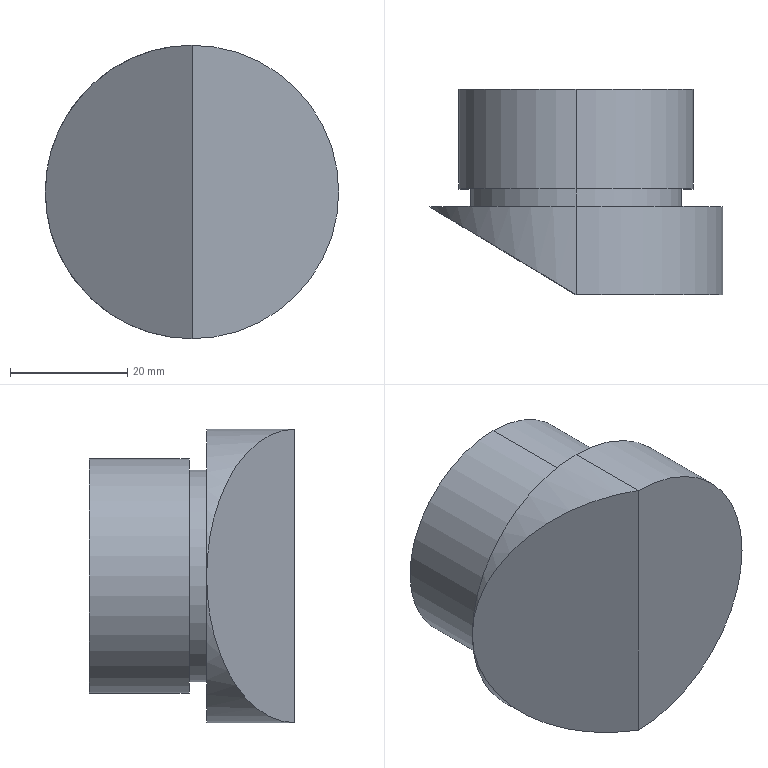Part | SolidWorks | features ICE 1, Revolution 1 | 1 solid | 12 faces | box 50 x 35 x 50 mm | volume 47619 mm3 | cylinder 7 | plane 5 | commonest cylinder face diameters 50 x3 36 x2 40 x2
STEP:
#1=CARTESIAN_POINT('',(0.,-2.175,18.));
#2=VERTEX_POINT('',#1);
#3=CARTESIAN_POINT('',(0.,-2.175,-18.));
#4=VERTEX_POINT('',#3);
#5=CARTESIAN_POINT('',(0.,-2.175,0.));
#6=DIRECTION('',(0.,1.,0.));
#7=DIRECTION('',(0.,0.,1.));
#8=AXIS2_PLACEMENT_3D('',#5,#6,#7);
#9=CIRCLE('',#8,18.);
#10=EDGE_CURVE('',#2,#4,#9,.T.);
#11=ORIENTED_EDGE('',*,*,#10,.T.);
#12=CARTESIAN_POINT('',(0.,0.8255,-18.));
#13=VERTEX_POINT('',#12);
#14=CARTESIAN_POINT('',(0.,13.712,-18.));
#15=DIRECTION('',(0.,1.,0.));
#16=VECTOR('',#15,1000.);
#17=LINE('',#14,#16);
#18=EDGE_CURVE('',#4,#13,#17,.T.);
#19=ORIENTED_EDGE('',*,*,#18,.T.);
#20=CARTESIAN_POINT('',(0.,0.8255,18.));
#21=VERTEX_POINT('',#20);
#22=CARTESIAN_POINT('',(0.,0.8255,0.));
#23=DIRECTION('',(0.,1.,0.));
#24=DIRECTION('',(0.,0.,1.));
#25=AXIS2_PLACEMENT_3D('',#22,#23,#24);
#26=CIRCLE('',#25,18.);
#27=EDGE_CURVE('',#21,#13,#26,.T.);
#28=ORIENTED_EDGE('',*,*,#27,.F.);
#29=CARTESIAN_POINT('',(0.,13.712,18.));
#30=DIRECTION('',(0.,1.,0.));
#31=VECTOR('',#30,1000.);
#32=LINE('',#29,#31);
#33=EDGE_CURVE('',#2,#21,#32,.T.);
#34=ORIENTED_EDGE('',*,*,#33,.F.);
#35=EDGE_LOOP('',(#11,#19,#28,#34));
#36=FACE_OUTER_BOUND('',#35,.T.);
#37=CARTESIAN_POINT('',(0.,13.712,0.));
#38=DIRECTION('',(0.,1.,0.));
#39=DIRECTION('',(0.,0.,1.));
#40=AXIS2_PLACEMENT_3D('',#37,#38,#39);
#41=CYLINDRICAL_SURFACE('',#40,18.);
#42=ADVANCED_FACE('',(#36),#41,.T.);
#43=CARTESIAN_POINT('',(0.,0.8255,20.));
#44=VERTEX_POINT('',#43);
#45=CARTESIAN_POINT('',(0.,0.8255,-20.));
#46=VERTEX_POINT('',#45);
#47=CARTESIAN_POINT('',(0.,0.8255,0.));
#48=DIRECTION('',(0.,1.,0.));
#49=DIRECTION('',(0.,0.,1.));
#50=AXIS2_PLACEMENT_3D('',#47,#48,#49);
#51=CIRCLE('',#50,20.);
#52=EDGE_CURVE('',#44,#46,#51,.T.);
#53=ORIENTED_EDGE('',*,*,#52,.T.);
#54=CARTESIAN_POINT('',(0.,17.825,-20.));
#55=VERTEX_POINT('',#54);
#56=CARTESIAN_POINT('',(0.,13.712,-20.));
#57=DIRECTION('',(0.,1.,0.));
#58=VECTOR('',#57,1000.);
#59=LINE('',#56,#58);
#60=EDGE_CURVE('',#46,#55,#59,.T.);
#61=ORIENTED_EDGE('',*,*,#60,.T.);
#62=CARTESIAN_POINT('',(0.,17.825,20.));
#63=VERTEX_POINT('',#62);
#64=CARTESIAN_POINT('',(0.,17.825,0.));
#65=DIRECTION('',(0.,1.,0.));
#66=DIRECTION('',(0.,0.,1.));
#67=AXIS2_PLACEMENT_3D('',#64,#65,#66);
#68=CIRCLE('',#67,20.);
#69=EDGE_CURVE('',#63,#55,#68,.T.);
#70=ORIENTED_EDGE('',*,*,#69,.F.);
#71=CARTESIAN_POINT('',(0.,13.712,20.));
#72=DIRECTION('',(0.,1.,0.));
#73=VECTOR('',#72,1000.);
#74=LINE('',#71,#73);
#75=EDGE_CURVE('',#44,#63,#74,.T.);
#76=ORIENTED_EDGE('',*,*,#75,.F.);
#77=EDGE_LOOP('',(#53,#61,#70,#76));
#78=FACE_OUTER_BOUND('',#77,.T.);
#79=CARTESIAN_POINT('',(0.,13.712,0.));
#80=DIRECTION('',(0.,1.,0.));
#81=DIRECTION('',(0.,0.,1.));
#82=AXIS2_PLACEMENT_3D('',#79,#80,#81);
#83=CYLINDRICAL_SURFACE('',#82,20.);
#84=ADVANCED_FACE('',(#78),#83,.T.);
#85=CARTESIAN_POINT('',(0.,-17.175,25.));
#86=VERTEX_POINT('',#85);
#87=CARTESIAN_POINT('',(0.,-17.175,-25.));
#88=VERTEX_POINT('',#87);
#89=CARTESIAN_POINT('',(0.,-17.175,0.));
#90=DIRECTION('',(0.,1.,0.));
#91=DIRECTION('',(0.,0.,1.));
#92=AXIS2_PLACEMENT_3D('',#89,#90,#91);
#93=CIRCLE('',#92,25.);
#94=EDGE_CURVE('',#86,#88,#93,.T.);
#95=ORIENTED_EDGE('',*,*,#94,.T.);
#96=CARTESIAN_POINT('',(0.,-2.175,-25.));
#97=VERTEX_POINT('',#96);
#98=CARTESIAN_POINT('',(0.,13.712,-25.));
#99=DIRECTION('',(0.,1.,0.));
#100=VECTOR('',#99,1000.);
#101=LINE('',#98,#100);
#102=EDGE_CURVE('',#88,#97,#101,.T.);
#103=ORIENTED_EDGE('',*,*,#102,.T.);
#104=CARTESIAN_POINT('',(0.,-2.175,25.));
#105=VERTEX_POINT('',#104);
#106=CARTESIAN_POINT('',(0.,-2.175,0.));
#107=DIRECTION('',(0.,1.,0.));
#108=DIRECTION('',(0.,0.,1.));
#109=AXIS2_PLACEMENT_3D('',#106,#107,#108);
#110=CIRCLE('',#109,25.);
#111=EDGE_CURVE('',#105,#97,#110,.T.);
#112=ORIENTED_EDGE('',*,*,#111,.F.);
#113=CARTESIAN_POINT('',(0.,13.712,25.));
#114=DIRECTION('',(0.,1.,0.));
#115=VECTOR('',#114,1000.);
#116=LINE('',#113,#115);
#117=EDGE_CURVE('',#86,#105,#116,.T.);
#118=ORIENTED_EDGE('',*,*,#117,.F.);
#119=EDGE_LOOP('',(#95,#103,#112,#118));
#120=FACE_OUTER_BOUND('',#119,.T.);
#121=CARTESIAN_POINT('',(0.,13.712,0.));
#122=DIRECTION('',(0.,1.,0.));
#123=DIRECTION('',(0.,0.,1.));
#124=AXIS2_PLACEMENT_3D('',#121,#122,#123);
#125=CYLINDRICAL_SURFACE('',#124,25.);
#126=ADVANCED_FACE('',(#120),#125,.T.);
#127=CARTESIAN_POINT('',(-25.,-2.175,0.));
#128=VERTEX_POINT('',#127);
#129=CARTESIAN_POINT('',(-25.,-2.175,0.));
#130=CARTESIAN_POINT('',(-25.,-2.175,14.645));
#131=CARTESIAN_POINT('',(-14.645,-8.388,25.));
#132=CARTESIAN_POINT('',(0.,-17.175,25.));
#133=(BOUNDED_CURVE()B_SPLINE_CURVE(3,(#129,#130,#131,#132),.UNSPECIFIED.,.F.,.F.)B_SPLINE_CURVE_WITH_KNOTS((4,4),(0.,1.571),.UNSPECIFIED.)CURVE()GEOMETRIC_REPRESENTATION_ITEM()RATIONAL_B_SPLINE_CURVE((1.,0.8047,0.8047,1.))REPRESENTATION_ITEM(''));
#134=EDGE_CURVE('',#128,#86,#133,.T.);
#135=ORIENTED_EDGE('',*,*,#134,.T.);
#136=ORIENTED_EDGE('',*,*,#117,.T.);
#137=CARTESIAN_POINT('',(0.,-2.175,0.));
#138=DIRECTION('',(0.,1.,0.));
#139=DIRECTION('',(0.,0.,1.));
#140=AXIS2_PLACEMENT_3D('',#137,#138,#139);
#141=CIRCLE('',#140,25.);
#142=EDGE_CURVE('',#128,#105,#141,.T.);
#143=ORIENTED_EDGE('',*,*,#142,.F.);
#144=EDGE_LOOP('',(#135,#136,#143));
#145=FACE_OUTER_BOUND('',#144,.T.);
#146=CARTESIAN_POINT('',(0.,13.712,0.));
#147=DIRECTION('',(0.,1.,0.));
#148=DIRECTION('',(0.,0.,1.));
#149=AXIS2_PLACEMENT_3D('',#146,#147,#148);
#150=CYLINDRICAL_SURFACE('',#149,25.);
#151=ADVANCED_FACE('',(#145),#150,.T.);
#152=ORIENTED_EDGE('',*,*,#102,.F.);
#153=CARTESIAN_POINT('',(0.,-17.175,-25.));
#154=CARTESIAN_POINT('',(-14.645,-8.388,-25.));
#155=CARTESIAN_POINT('',(-25.,-2.175,-14.645));
#156=CARTESIAN_POINT('',(-25.,-2.175,0.));
#157=(BOUNDED_CURVE()B_SPLINE_CURVE(3,(#153,#154,#155,#156),.UNSPECIFIED.,.F.,.F.)B_SPLINE_CURVE_WITH_KNOTS((4,4),(4.712,6.283),.UNSPECIFIED.)CURVE()GEOMETRIC_REPRESENTATION_ITEM()RATIONAL_B_SPLINE_CURVE((1.,0.8047,0.8047,1.))REPRESENTATION_ITEM(''));
#158=EDGE_CURVE('',#88,#128,#157,.T.);
#159=ORIENTED_EDGE('',*,*,#158,.T.);
#160=CARTESIAN_POINT('',(0.,-2.175,0.));
#161=DIRECTION('',(0.,1.,0.));
#162=DIRECTION('',(0.,0.,1.));
#163=AXIS2_PLACEMENT_3D('',#160,#161,#162);
#164=CIRCLE('',#163,25.);
#165=EDGE_CURVE('',#97,#128,#164,.T.);
#166=ORIENTED_EDGE('',*,*,#165,.F.);
#167=EDGE_LOOP('',(#152,#159,#166));
#168=FACE_OUTER_BOUND('',#167,.T.);
#169=CARTESIAN_POINT('',(0.,13.712,0.));
#170=DIRECTION('',(0.,1.,0.));
#171=DIRECTION('',(0.,0.,1.));
#172=AXIS2_PLACEMENT_3D('',#169,#170,#171);
#173=CYLINDRICAL_SURFACE('',#172,25.);
#174=ADVANCED_FACE('',(#168),#173,.T.);
#175=CARTESIAN_POINT('',(0.,-17.175,-25.));
#176=DIRECTION('',(0.,0.,1.));
#177=VECTOR('',#176,1000.);
#178=LINE('',#175,#177);
#179=EDGE_CURVE('',#88,#86,#178,.T.);
#180=ORIENTED_EDGE('',*,*,#179,.F.);
#181=ORIENTED_EDGE('',*,*,#94,.F.);
#182=EDGE_LOOP('',(#180,#181));
#183=FACE_OUTER_BOUND('',#182,.T.);
#184=CARTESIAN_POINT('',(0.,-17.175,0.));
#185=DIRECTION('',(0.,1.,0.));
#186=DIRECTION('',(0.,0.,1.));
#187=AXIS2_PLACEMENT_3D('',#184,#185,#186);
#188=PLANE('',#187);
#189=ADVANCED_FACE('',(#183),#188,.F.);
#190=ORIENTED_EDGE('',*,*,#69,.T.);
#191=CARTESIAN_POINT('',(0.,17.825,0.));
#192=DIRECTION('',(0.,1.,0.));
#193=DIRECTION('',(0.,0.,1.));
#194=AXIS2_PLACEMENT_3D('',#191,#192,#193);
#195=CIRCLE('',#194,20.);
#196=EDGE_CURVE('',#55,#63,#195,.T.);
#197=ORIENTED_EDGE('',*,*,#196,.T.);
#198=EDGE_LOOP('',(#190,#197));
#199=FACE_OUTER_BOUND('',#198,.T.);
#200=CARTESIAN_POINT('',(0.,17.825,0.));
#201=DIRECTION('',(0.,1.,0.));
#202=DIRECTION('',(0.,0.,1.));
#203=AXIS2_PLACEMENT_3D('',#200,#201,#202);
#204=PLANE('',#203);
#205=ADVANCED_FACE('',(#199),#204,.T.);
#206=ORIENTED_EDGE('',*,*,#60,.F.);
#207=CARTESIAN_POINT('',(0.,0.8255,0.));
#208=DIRECTION('',(0.,1.,0.));
#209=DIRECTION('',(0.,0.,1.));
#210=AXIS2_PLACEMENT_3D('',#207,#208,#209);
#211=CIRCLE('',#210,20.);
#212=EDGE_CURVE('',#46,#44,#211,.T.);
#213=ORIENTED_EDGE('',*,*,#212,.T.);
#214=ORIENTED_EDGE('',*,*,#75,.T.);
#215=ORIENTED_EDGE('',*,*,#196,.F.);
#216=EDGE_LOOP('',(#206,#213,#214,#215));
#217=FACE_OUTER_BOUND('',#216,.T.);
#218=CARTESIAN_POINT('',(0.,13.712,0.));
#219=DIRECTION('',(0.,1.,0.));
#220=DIRECTION('',(0.,0.,1.));
#221=AXIS2_PLACEMENT_3D('',#218,#219,#220);
#222=CYLINDRICAL_SURFACE('',#221,20.);
#223=ADVANCED_FACE('',(#217),#222,.T.);
#224=ORIENTED_EDGE('',*,*,#52,.F.);
#225=ORIENTED_EDGE('',*,*,#212,.F.);
#226=EDGE_LOOP('',(#224,#225));
#227=FACE_OUTER_BOUND('',#226,.T.);
#228=ORIENTED_EDGE('',*,*,#27,.T.);
#229=CARTESIAN_POINT('',(0.,0.8255,0.));
#230=DIRECTION('',(0.,1.,0.));
#231=DIRECTION('',(0.,0.,1.));
#232=AXIS2_PLACEMENT_3D('',#229,#230,#231);
#233=CIRCLE('',#232,18.);
#234=EDGE_CURVE('',#13,#21,#233,.T.);
#235=ORIENTED_EDGE('',*,*,#234,.T.);
#236=EDGE_LOOP('',(#228,#235));
#237=FACE_BOUND('',#236,.T.);
#238=CARTESIAN_POINT('',(0.,0.8255,0.));
#239=DIRECTION('',(0.,1.,0.));
#240=DIRECTION('',(0.,0.,1.));
#241=AXIS2_PLACEMENT_3D('',#238,#239,#240);
#242=PLANE('',#241);
#243=ADVANCED_FACE('',(#227,#237),#242,.F.);
#244=ORIENTED_EDGE('',*,*,#18,.F.);
#245=CARTESIAN_POINT('',(0.,-2.175,0.));
#246=DIRECTION('',(0.,1.,0.));
#247=DIRECTION('',(0.,0.,1.));
#248=AXIS2_PLACEMENT_3D('',#245,#246,#247);
#249=CIRCLE('',#248,18.);
#250=EDGE_CURVE('',#4,#2,#249,.T.);
#251=ORIENTED_EDGE('',*,*,#250,.T.);
#252=ORIENTED_EDGE('',*,*,#33,.T.);
#253=ORIENTED_EDGE('',*,*,#234,.F.);
#254=EDGE_LOOP('',(#244,#251,#252,#253));
#255=FACE_OUTER_BOUND('',#254,.T.);
#256=CARTESIAN_POINT('',(0.,13.712,0.));
#257=DIRECTION('',(0.,1.,0.));
#258=DIRECTION('',(0.,0.,1.));
#259=AXIS2_PLACEMENT_3D('',#256,#257,#258);
#260=CYLINDRICAL_SURFACE('',#259,18.);
#261=ADVANCED_FACE('',(#255),#260,.T.);
#262=ORIENTED_EDGE('',*,*,#142,.T.);
#263=ORIENTED_EDGE('',*,*,#111,.T.);
#264=ORIENTED_EDGE('',*,*,#165,.T.);
#265=EDGE_LOOP('',(#262,#263,#264));
#266=FACE_OUTER_BOUND('',#265,.T.);
#267=ORIENTED_EDGE('',*,*,#10,.F.);
#268=ORIENTED_EDGE('',*,*,#250,.F.);
#269=EDGE_LOOP('',(#267,#268));
#270=FACE_BOUND('',#269,.T.);
#271=CARTESIAN_POINT('',(0.,-2.175,0.));
#272=DIRECTION('',(0.,1.,0.));
#273=DIRECTION('',(0.,0.,1.));
#274=AXIS2_PLACEMENT_3D('',#271,#272,#273);
#275=PLANE('',#274);
#276=ADVANCED_FACE('',(#266,#270),#275,.T.);
#277=ORIENTED_EDGE('',*,*,#158,.F.);
#278=ORIENTED_EDGE('',*,*,#179,.T.);
#279=ORIENTED_EDGE('',*,*,#134,.F.);
#280=EDGE_LOOP('',(#277,#278,#279));
#281=FACE_OUTER_BOUND('',#280,.T.);
#282=CARTESIAN_POINT('',(-7.577,-12.628,-25.));
#283=DIRECTION('',(-0.5145,-0.8575,0.));
#284=DIRECTION('',(0.8575,-0.5145,0.));
#285=AXIS2_PLACEMENT_3D('',#282,#283,#284);
#286=PLANE('',#285);
#287=ADVANCED_FACE('',(#281),#286,.T.);
#288=CLOSED_SHELL('',(#42,#84,#126,#151,#174,#189,#205,#223,#243,#261,#276,#287));
#289=MANIFOLD_SOLID_BREP('',#288);
#290=CARTESIAN_POINT('',(0.,0.,0.));
#291=DIRECTION('',(0.,0.,1.));
#292=DIRECTION('',(1.,0.,0.));
#293=AXIS2_PLACEMENT_3D('',#290,#291,#292);
#294=(LENGTH_UNIT()NAMED_UNIT(*)SI_UNIT(.MILLI.,.METRE.));
#295=UNCERTAINTY_MEASURE_WITH_UNIT(LENGTH_MEASURE(0.00001),#294,'','');
#296=(NAMED_UNIT(*)PLANE_ANGLE_UNIT()SI_UNIT($,.RADIAN.));
#297=(NAMED_UNIT(*)SI_UNIT($,.STERADIAN.)SOLID_ANGLE_UNIT());
#298=(GEOMETRIC_REPRESENTATION_CONTEXT(3)GLOBAL_UNCERTAINTY_ASSIGNED_CONTEXT((#295))GLOBAL_UNIT_ASSIGNED_CONTEXT((#294,#296,#297))REPRESENTATION_CONTEXT('',''));
#299=ADVANCED_BREP_SHAPE_REPRESENTATION('',(#289,#293),#298);